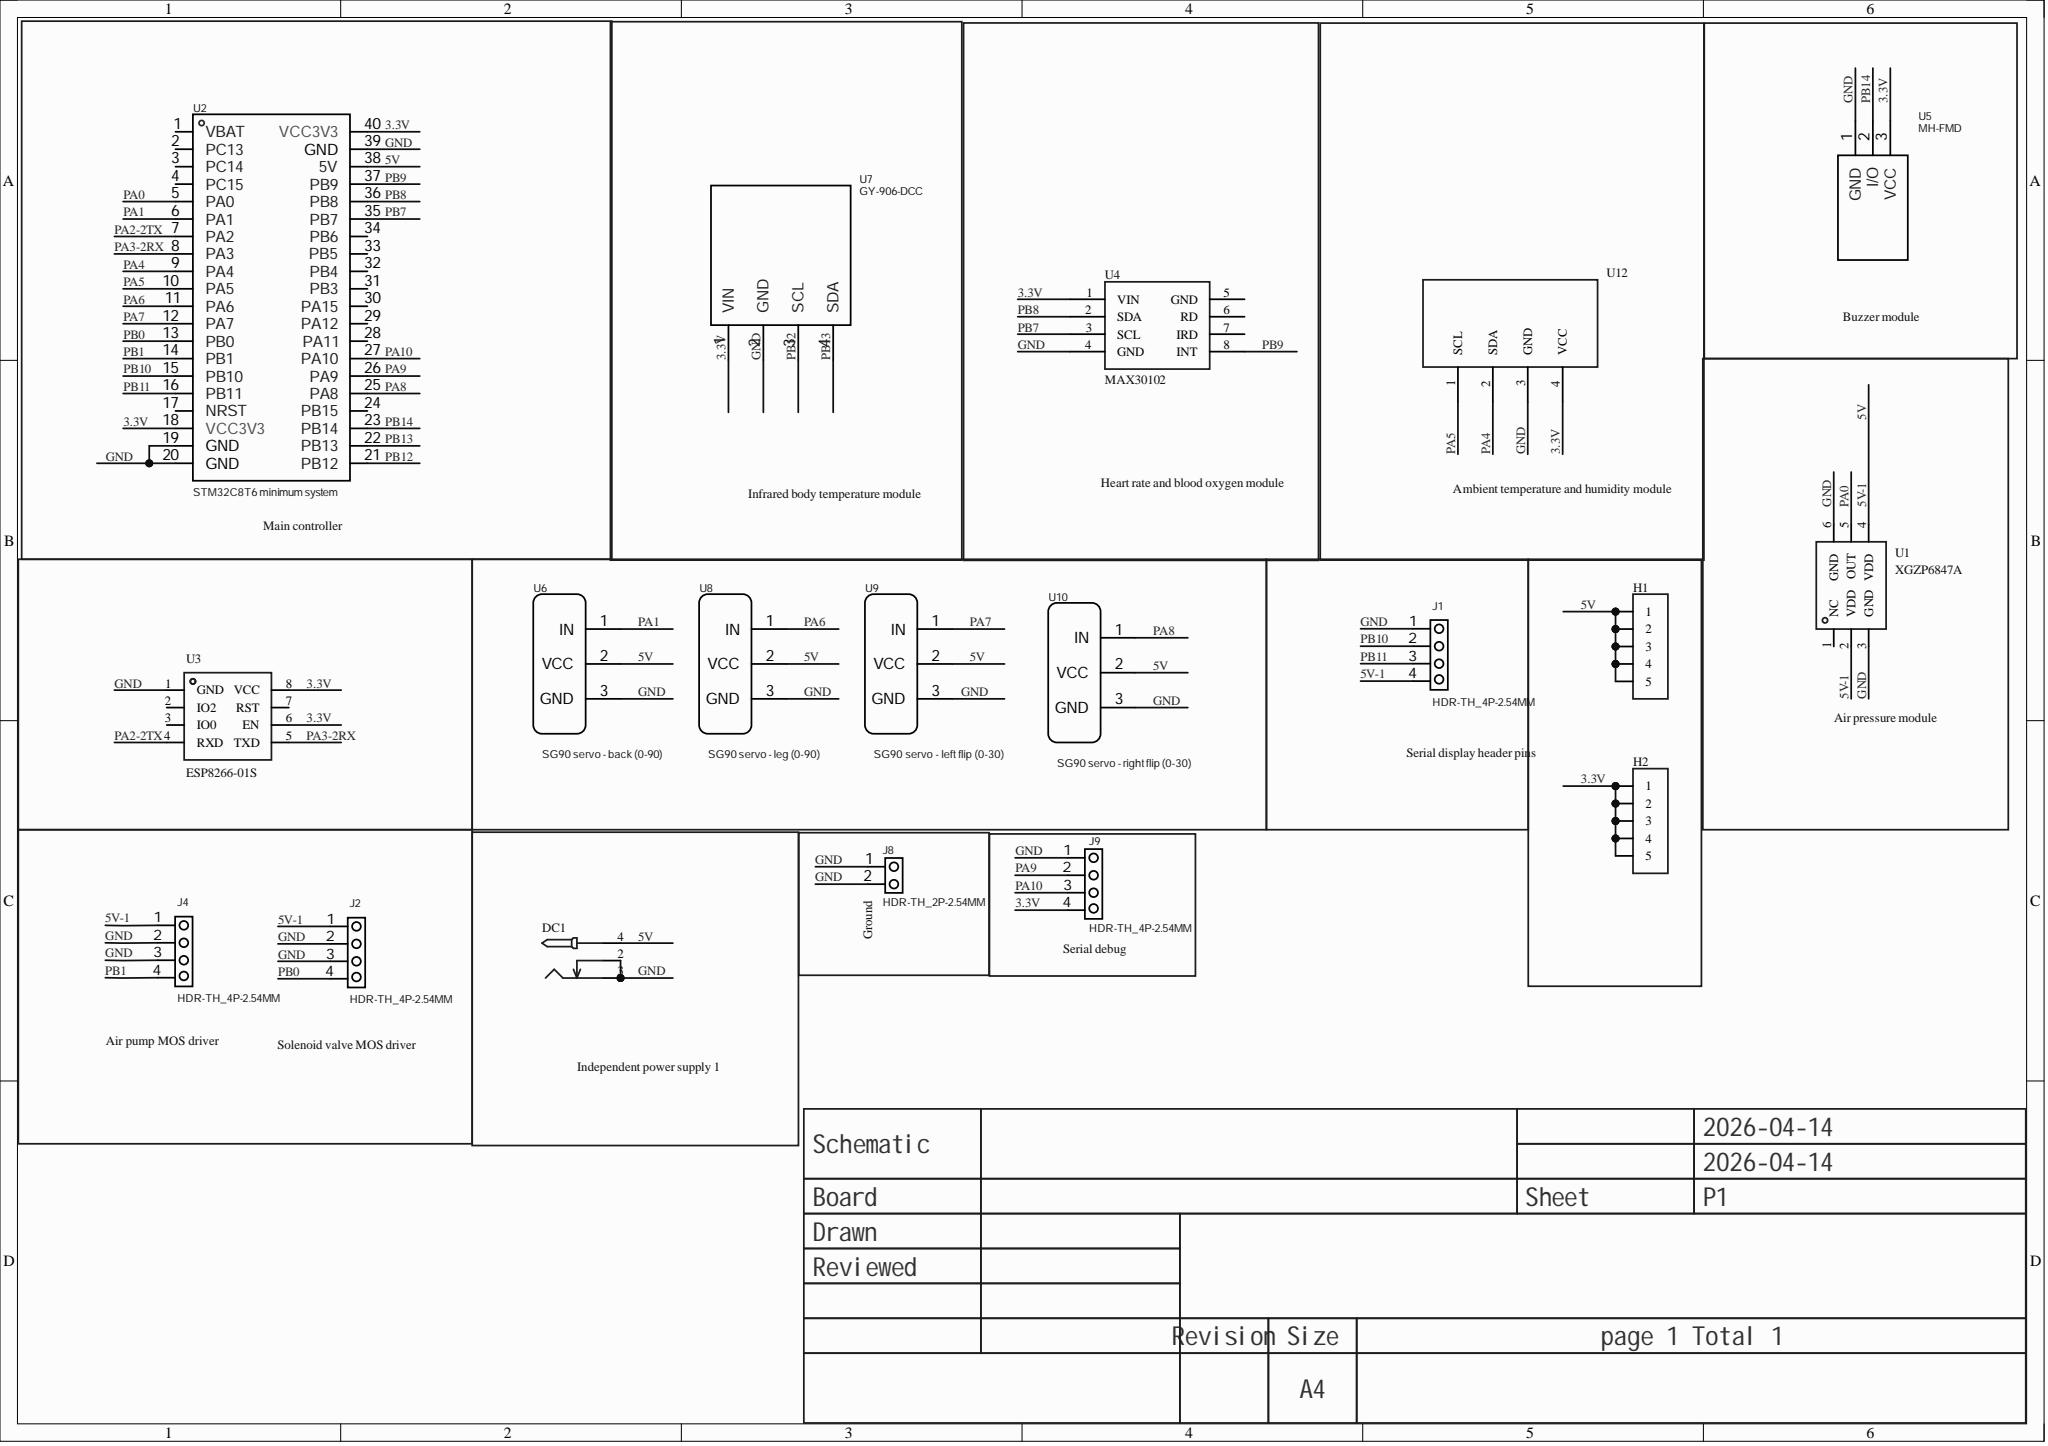Circuit board | Altium Designer | 19 parts | 24 nets
Bill of materials:
Comment,Description,Designator,Footprint,LibRef,Quantity
"","","DC1","DC-2.0","DC-005_2.0","1"
"","","H1, H2","HDR-TH_5P-P2.54-V-F","HDR-F_2.54_1x5P","2"
"HDR-TH_4P-2.54MM","","J1, J2, J4, J9","HDR-TH_4P-2.54MM","HDR-TH_4P-2.54MM","4"
"HDR-TH_2P-2.54MM","","J8","HDR-TH_2P-2.54MM","HDR-TH_2P-2.54MM","1"
"XGZP6847A","","U1","SENSOR-TH_XGZP6847A","XGZP6847A","1"
"STM32C8T6 minimum system","","U2","STM32F103C8T6最小系统插座","STM32C8T6最小系统","1"
"ESP8266-01S","","U3","WIFIM-TH_ESP8266-01S","ESP8266-01S","1"
"MAX30102","","U4","MAX30102","MAX30102","1"
"MH-FMD","","U5","MH-FMD","MH-FMD","1"
"SG90 servo - back (0-90)","","U6","SG90","SG90舵机","1"
"GY-906-DCC","","U7","GY-906-DCC","GY-906-DCC","1"
"SG90 servo - leg (0-90)","","U8","SG90","SG90舵机","1"
"SG90 servo - left flip (0-30)","","U9","SG90","SG90舵机","1"
"SG90 servo - right flip (0-30)","","U10","SG90","SG90舵机","1"
"","","U12","SHT30","SHT30","1"
Netlist (Protel format):
[
DC1
DC-2.0




]
[
H1
HDR-TH_5P-P2.54-V-F




]
[
H2
HDR-TH_5P-P2.54-V-F




]
[
J1
HDR-TH_4P-2.54MM
HDR-TH_4P-2.54MM



]
[
J2
HDR-TH_4P-2.54MM
HDR-TH_4P-2.54MM



]
[
J4
HDR-TH_4P-2.54MM
HDR-TH_4P-2.54MM



]
[
J8
HDR-TH_2P-2.54MM
HDR-TH_2P-2.54MM



]
[
J9
HDR-TH_4P-2.54MM
HDR-TH_4P-2.54MM



]
[
U1
SENSOR-TH_XGZP6847A
XGZP6847A



]
[
U2
STM32F103C8T6最小系统插座
STM32C8T6 minimum system



]
[
U3
WIFIM-TH_ESP8266-01S
ESP8266-01S



]
[
U4
MAX30102
MAX30102



]
[
U5
MH-FMD
MH-FMD



]
[
U6
SG90
SG90 servo - back (0-90)



]
[
U7
GY-906-DCC
GY-906-DCC



]
[
U8
SG90
SG90 servo - leg (0-90)



]
[
U9
SG90
SG90 servo - left flip (0-30)



]
[
U10
SG90
SG90 servo - right flip (0-30)



]
[
U12
SHT30




]
(
PB14
U2-23
U5-2
)
(
PB13
U2-22
U7-4
)
(
PB12
U2-21
U7-3
)
(
PB11
J1-3
U2-16
)
(
PB10
J1-2
U2-15
)
(
PB9
U2-37
U4-8
)
(
PB8
U2-36
U4-2
)
(
PB7
U2-35
U4-3
)
(
PB1
J4-4
U2-14
)
(
PB0
J2-4
U2-13
)
(
PA10
J9-3
U2-27
)
(
PA9
J9-2
U2-26
)
(
PA8
U2-25
U10-1
)
(
PA7
U2-12
U9-1
)
(
PA6
U2-11
U8-1
)
(
PA5
U2-10
U12-1
)
(
PA4
U2-9
U12-2
)
(
PA3-2RX
U2-8
U3-5
)
(
PA2-2TX
U2-7
U3-4
)
(
PA1
U2-6
U6-1
)
(
PA0
U1-5
U2-5
)
(
GND
DC1-2
DC1-3
J1-1
J2-2
J2-3
J4-2
J4-3
J8-1
J8-2
J9-1
U1-3
U1-6
U2-19
U2-20
U2-39
U3-1
U4-4
U5-1
U6-3
U7-2
U8-3
U9-3
U10-3
U12-3
)
(
5V
DC1-4
H1-1
H1-2
H1-3
H1-4
H1-5
J1-4
J2-1
J4-1
U1-2
U1-4
U2-38
U6-2
U8-2
U9-2
U10-2
)
(
3.3V
H2-1
H2-2
H2-3
H2-4
H2-5
J9-4
U2-18
U2-40
U3-6
U3-8
U4-1
U5-3
U7-1
U12-4
)